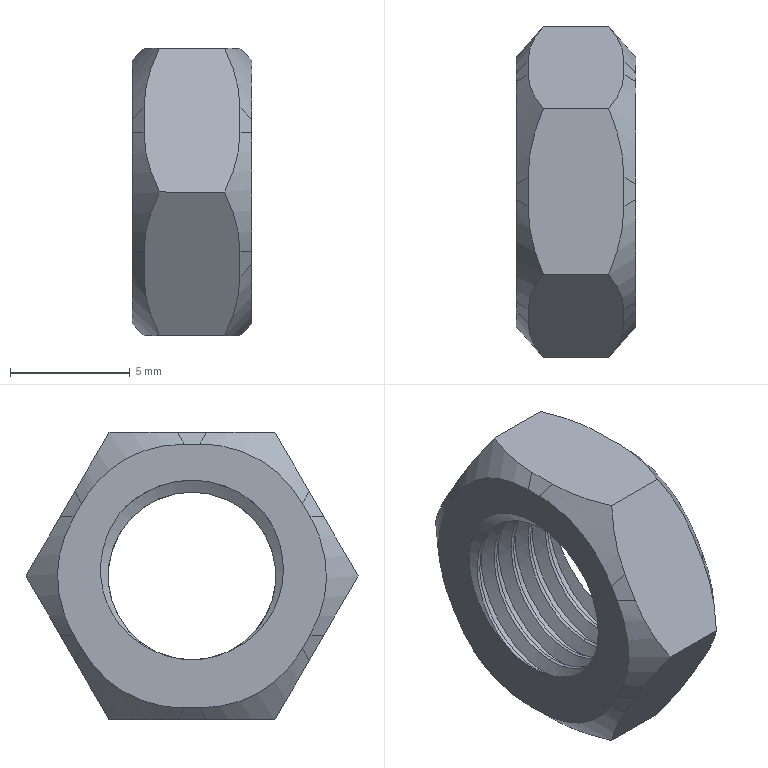Part | SolidWorks | features BaseBody 1 | 1 solid | 58 faces | box 5 x 13.856 x 12 mm | volume 377.79 mm3 | cylinder 36 | plane 20 | spline 2 | commonest cylinder face diameters 7 x12 8 x12 14 x12